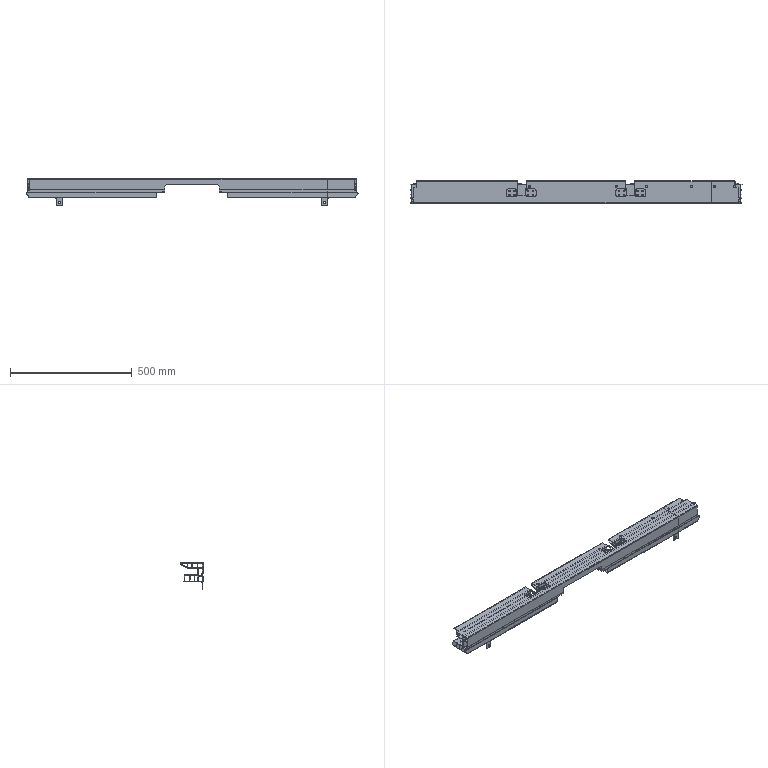NC program | NX | posted with a generic post | part box 1365 x 90.95 x 108.501 mm
Lines 1 to 1032 of 23380:
N10 G17 G21 G94 G90
(FLOOR_WALL_COPY_COPY , TOOL : D10)
N12 T10 M6
N14 G54
N16 G17 G0 G90 X-649.118 Y38.719 B0. C0. S6000 M3
N18 G43 Z30. H10
N20 Z0.524
N22 G94 G1 Z-0.976 F1000.
N24 X-648.541 Y39.719
N26 G2 X-647.675 Y40.219 R1.
N28 G1 X-622.6 F2500.
N30 Y44.
N32 G3 X-625. Y46.4 R2.4
N34 G1 X-658.759
N36 G2 X-658.96 Y46.442 R0.5
N38 G1 X-660.602 Y47.163
N40 X-660.976 Y47.3
N42 X-665.955 Y48.486
N44 G2 X-666.339 Y48.973 R0.5
N46 G1 Y57.612
N48 G2 X-665.945 Y58.1 R0.5
N50 G1 X-664.104 Y58.5
N52 X-672.75
N54 Y40.219
N56 X-647.675
N58 G2 X-646.809 Y39.719 R1.
N60 G1 X-646.232 Y38.719
N62 Z0.524
N64 G0 X-623.698
N66 G1 Z-0.976 F1000.
N68 X-622.6 Y39.353
N70 G3 X-622.1 Y40.219 R1.
N72 G1 Y44. F2500.
N74 G3 X-625. Y46.9 R2.9
N76 G1 X-658.759
N78 X-660.415 Y47.627
N80 X-660.832 Y47.779
N82 X-665.839 Y48.973
N84 Y57.612
N86 X-661.885 Y58.47
N88 G3 X-661.145 Y59.142 R1.
N90 G1 X-660.55 Y61.
N92 Z0.524
N94 G0 Z30.
N96 X-662.961 Y47.773
N98 Z0.524
N100 G1 X-666.007 Y48.502 Z0.36 F1000.
N102 X-666.045 Y48.515 Z0.358
N104 X-666.234 Y48.619 Z0.346
N106 X-666.339 Y48.797 Z0.335
N108 Y57.727 Z-0.133
N110 X-666.212 Y57.988 Z-0.148
N112 X-666.117 Y58.063 Z-0.154
N114 X-664.104 Y58.5 Z-0.262
N116 X-672.75 Z-0.715
N118 Y39.764 Z-1.697
N120 X-667.885 Z-1.952
N122 Y44.264
N124 X-667.52 F2500.
N126 G2 X-668.25 Y44.592 R5.
N128 G1 Y44.264
N130 X-667.885
N132 Y39.764
N134 X-622.6
N136 Y44.
N138 G3 X-625. Y46.4 R2.4
N140 G1 X-658.759
N142 G2 X-658.96 Y46.442 R0.5
N144 G1 X-660.602 Y47.163
N146 X-660.976 Y47.3
N148 X-666.007 Y48.502
N150 X-666.08 Y48.535
N152 G2 X-666.339 Y48.973 R0.5
N154 G1 Y57.612
N156 G2 X-665.945 Y58.1 R0.5
N158 G1 X-664.104 Y58.5
N160 X-672.75
N162 Y39.764
N164 X-667.885
N166 G2 X-667.019 Y39.264 R1.
N168 G1 X-666.442 Y38.264
N170 Z-0.452
N172 G0 X-623.698
N174 G1 Z-1.952 F1000.
N176 X-622.6 Y38.898
N178 G3 X-622.1 Y39.764 R1.
N180 G1 Y44. F2500.
N182 G3 X-625. Y46.9 R2.9
N184 G1 X-658.759
N186 X-660.415 Y47.627
N188 X-660.832 Y47.779
N190 X-665.839 Y48.973
N192 Y57.612
N194 X-661.885 Y58.47
N196 G3 X-661.145 Y59.142 R1.
N198 G1 X-660.55 Y61.
N200 Z-0.452
N202 G0 Z30.
N204 X-664.27 Y48.085
N206 Z-0.452
N208 G1 X-666.021 Y48.502 Z-0.546 F1000.
N210 X-666.234 Y48.619 Z-0.559
N212 X-666.339 Y48.797 Z-0.57
N214 Y57.727 Z-1.038
N216 X-666.212 Y57.988 Z-1.053
N218 X-666.117 Y58.063 Z-1.06
N220 X-664.104 Y58.5 Z-1.168
N222 X-672.75 Z-1.621
N224 Y39.309 Z-2.626
N226 X-666.995 Z-2.928
N228 Y43.809
N230 X-665.739 F2500.
N232 X-666.998 Y44.109
N234 G2 X-668.25 Y44.592 R5.
N236 G1 Y43.809
N238 X-666.995
N240 Y39.309
N242 X-622.6
N244 Y44.
N246 G3 X-625. Y46.4 R2.4
N248 G1 X-658.759
N250 G2 X-658.96 Y46.442 R0.5
N252 G1 X-660.602 Y47.163
N254 X-660.976 Y47.3
N256 X-665.955 Y48.486
N258 G2 X-666.339 Y48.973 R0.5
N260 G1 Y57.612
N262 G2 X-665.945 Y58.1 R0.5
N264 G1 X-664.104 Y58.5
N266 X-672.75
N268 Y39.309
N270 X-666.995
N272 G2 X-666.129 Y38.809 R1.
N274 G1 X-665.551 Y37.809
N276 Z-1.428
N278 G0 X-623.698
N280 G1 Z-2.928 F1000.
N282 X-622.6 Y38.443
N284 G3 X-622.1 Y39.309 R1.
N286 G1 Y44. F2500.
N288 G3 X-625. Y46.9 R2.9
N290 G1 X-658.759
N292 X-660.415 Y47.627
N294 X-660.832 Y47.779
N296 X-665.839 Y48.973
N298 Y57.612
N300 X-661.885 Y58.47
N302 G3 X-661.145 Y59.142 R1.
N304 G1 X-660.55 Y61.
N306 Z-1.428
N308 G0 Z30.
N310 X-665.665 Y43.791
N312 Z-1.428
N314 G1 X-667.532 Y44.236 Z-1.529 F1000.
N316 X-667.769 Y44.328 Z-1.542
N318 X-668.25 Y44.592 Z-1.571
N320 Y43.354 Z-1.636
N322 X-663.83 Z-1.867
N324 X-666.998 Y44.109 Z-2.038
N326 X-667.532 Y44.236 Z-2.067
N328 X-667.769 Y44.328 Z-2.08
N330 X-668.25 Y44.592 Z-2.109
N332 Y43.354 Z-2.174
N334 X-663.83 Z-2.405
N336 X-666.998 Y44.109 Z-2.576
N338 X-667.532 Y44.236 Z-2.605
N340 X-667.769 Y44.328 Z-2.618
N342 X-668.25 Y44.592 Z-2.647
N344 Y43.354 Z-2.712
N346 X-663.83 Z-2.944
N348 X-666.998 Y44.109 Z-3.114
N350 X-667.532 Y44.236 Z-3.143
N352 X-667.769 Y44.328 Z-3.156
N354 X-668.25 Y44.592 Z-3.185
N356 Y43.354 Z-3.25
N358 X-663.83 Z-3.482
N360 X-666.998 Y44.109 Z-3.652
N362 X-667.532 Y44.236 Z-3.681
N364 X-667.769 Y44.328 Z-3.694
N366 X-668.25 Y44.592 Z-3.723
N368 Y43.354 Z-3.788
N370 X-666.04 Z-3.904
N372 X-663.83 F2500.
N374 X-666.998 Y44.109
N376 G2 X-668.25 Y44.592 R5.
N378 G1 Y43.354
N380 X-666.04
N382 Y38.854
N384 X-622.6
N386 Y44.
N388 G3 X-625. Y46.4 R2.4
N390 G1 X-658.759
N392 G2 X-658.96 Y46.442 R0.5
N394 G1 X-660.602 Y47.163
N396 X-660.976 Y47.3
N398 X-665.955 Y48.486
N400 G2 X-666.339 Y48.973 R0.5
N402 G1 Y57.612
N404 G2 X-665.945 Y58.1 R0.5
N406 G1 X-664.104 Y58.5
N408 X-672.75
N410 Y38.854
N412 X-666.04
N414 G2 X-665.174 Y38.354 R1.
N416 G1 X-664.596 Y37.354
N418 Z-2.404
N420 G0 X-623.698
N422 G1 Z-3.904 F1000.
N424 X-622.6 Y37.988
N426 G3 X-622.1 Y38.854 R1.
N428 G1 Y44. F2500.
N430 G3 X-625. Y46.9 R2.9
N432 G1 X-658.759
N434 X-660.415 Y47.627
N436 X-660.832 Y47.779
N438 X-665.839 Y48.973
N440 Y57.612
N442 X-661.885 Y58.47
N444 G3 X-661.145 Y59.142 R1.
N446 G1 X-660.55 Y61.
N448 Z-2.404
N450 G0 Z30.
N452 X-668.25 Y44.222
N454 Z-2.404
N456 G1 Y42.899 Z-2.473 F1000.
N458 X-662.082 Z-2.797
N460 X-662.275 Y42.983 Z-2.808
N462 X-666.998 Y44.109 Z-3.062
N464 X-667.532 Y44.236 Z-3.091
N466 X-667.769 Y44.328 Z-3.104
N468 X-668.25 Y44.592 Z-3.133
N470 Y42.899 Z-3.222
N472 X-662.082 Z-3.545
N474 X-662.275 Y42.983 Z-3.556
N476 X-666.998 Y44.109 Z-3.81
N478 X-667.532 Y44.236 Z-3.839
N480 X-667.769 Y44.328 Z-3.852
N482 X-668.25 Y44.592 Z-3.881
N484 Y42.899 Z-3.97
N486 X-662.082 Z-4.293
N488 X-662.275 Y42.983 Z-4.304
N490 X-666.998 Y44.109 Z-4.559
N492 X-667.532 Y44.236 Z-4.587
N494 X-667.769 Y44.328 Z-4.601
N496 X-668.25 Y44.592 Z-4.629
N498 Y42.899 Z-4.718
N500 X-665.166 Z-4.88
N502 X-662.082 F2500.
N504 X-662.275 Y42.983
N506 X-666.998 Y44.109
N508 G2 X-668.25 Y44.592 R5.
N510 G1 Y42.899
N512 X-665.166
N514 Y38.399
N516 X-622.6
N518 Y44.
N520 G3 X-625. Y46.4 R2.4
N522 G1 X-658.759
N524 G2 X-658.96 Y46.442 R0.5
N526 G1 X-660.976 Y47.3
N528 X-665.955 Y48.486
N530 G2 X-666.339 Y48.973 R0.5
N532 G1 Y57.612
N534 G2 X-665.945 Y58.1 R0.5
N536 G1 X-664.104 Y58.5
N538 X-672.75
N540 Y38.399
N542 X-665.166
N544 G2 X-664.3 Y37.899 R1.
N546 G1 X-663.723 Y36.899
N548 Z-3.38
N550 G0 X-623.698
N552 G1 Z-4.88 F1000.
N554 X-622.6 Y37.533
N556 G3 X-622.1 Y38.399 R1.
N558 G1 Y44. F2500.
N560 G3 X-625. Y46.9 R2.9
N562 G1 X-658.759
N564 X-660.415 Y47.627
N566 X-660.832 Y47.779
N568 X-665.839 Y48.973
N570 Y57.612
N572 X-661.885 Y58.47
N574 G3 X-661.145 Y59.142 R1.
N576 G1 X-660.55 Y61.
N578 Z-3.38
N580 G0 Z30.
N582 X-661.184 Y42.444
N584 Z-3.38
N586 G1 X-661.046 Z-3.387 F1000.
N588 X-662.275 Y42.983 Z-3.457
N590 X-666.998 Y44.109 Z-3.712
N592 X-667.532 Y44.236 Z-3.741
N594 X-667.769 Y44.328 Z-3.754
N596 X-668.25 Y44.592 Z-3.783
N598 Y42.444 Z-3.895
N600 X-661.046 Z-4.273
N602 X-662.275 Y42.983 Z-4.343
N604 X-666.998 Y44.109 Z-4.598
N606 X-667.532 Y44.236 Z-4.627
N608 X-667.769 Y44.328 Z-4.64
N610 X-668.25 Y44.592 Z-4.669
N612 Y42.444 Z-4.781
N614 X-661.046 Z-5.159
N616 X-662.275 Y42.983 Z-5.229
N618 X-666.998 Y44.109 Z-5.484
N620 X-667.532 Y44.236 Z-5.512
N622 X-667.769 Y44.328 Z-5.526
N624 X-668.25 Y44.592 Z-5.554
N626 Y42.444 Z-5.667
N628 X-664.648 Z-5.856
N630 X-661.046 F2500.
N632 X-662.275 Y42.983
N634 X-666.998 Y44.109
N636 G2 X-668.25 Y44.592 R5.
N638 G1 Y42.444
N640 X-664.648
N642 Y37.944
N644 X-622.6
N646 Y44.
N648 G3 X-625. Y46.4 R2.4
N650 G1 X-658.759
N652 G2 X-658.96 Y46.442 R0.5
N654 G1 X-660.976 Y47.3
N656 X-665.955 Y48.486
N658 G2 X-666.339 Y48.973 R0.5
N660 G1 Y57.612
N662 G2 X-665.945 Y58.1 R0.5
N664 G1 X-664.104 Y58.5
N666 X-672.75
N668 Y37.944
N670 X-664.648
N672 G2 X-663.782 Y37.444 R1.
N674 G1 X-663.205 Y36.444
N676 Z-4.356
N678 G0 X-623.698
N680 G1 Z-5.856 F1000.
N682 X-622.6 Y37.078
N684 G3 X-622.1 Y37.944 R1.
N686 G1 Y44. F2500.
N688 G3 X-625. Y46.9 R2.9
N690 G1 X-658.759
N692 X-660.415 Y47.627
N694 X-660.832 Y47.779
N696 X-665.839 Y48.973
N698 Y57.612
N700 X-661.885 Y58.47
N702 G3 X-661.145 Y59.142 R1.
N704 G1 X-660.55 Y61.
N706 Z-4.356
N708 G0 Z30.
N710 X-668.182 Y44.555
N712 Z-4.356
N714 G1 X-668.25 Y44.592 Z-4.36 F1000.
N716 Y41.988 Z-4.496
N718 X-659.695 Z-4.945
N720 X-660.234 Y42.091 Z-4.973
N722 X-660.267 Y42.101 Z-4.975
N724 X-662.275 Y42.983 Z-5.09
N726 X-666.998 Y44.109 Z-5.345
N728 X-667.532 Y44.236 Z-5.373
N730 X-667.769 Y44.328 Z-5.387
N732 X-668.25 Y44.592 Z-5.415
N734 Y41.988 Z-5.552
N736 X-659.695 Z-6.
N738 X-660.234 Y42.091 Z-6.029
N740 X-660.267 Y42.101 Z-6.031
N742 X-662.275 Y42.983 Z-6.146
N744 X-666.998 Y44.109 Z-6.4
N746 X-667.532 Y44.236 Z-6.429
N748 X-667.769 Y44.328 Z-6.442
N750 X-668.25 Y44.592 Z-6.471
N752 Y41.988 Z-6.608
N754 X-663.973 Z-6.832
N756 X-659.695 F2500.
N758 G2 X-660.769 Y42.322 R5.
N760 G1 X-662.275 Y42.983
N762 X-666.998 Y44.109
N764 G2 X-668.25 Y44.592 R5.
N766 G1 Y41.988
N768 X-663.973
N770 Y37.488
N772 X-622.6
N774 Y44.
N776 G3 X-625. Y46.4 R2.4
N778 G1 X-658.759
N780 G2 X-658.96 Y46.442 R0.5
N782 G1 X-660.602 Y47.163
N784 X-660.976 Y47.3
N786 X-665.955 Y48.486
N788 G2 X-666.339 Y48.973 R0.5
N790 G1 Y57.612
N792 G2 X-665.945 Y58.1 R0.5
N794 G1 X-664.104 Y58.5
N796 X-672.75
N798 Y37.488
N800 X-663.973
N802 G2 X-663.107 Y36.988 R1.
N804 G1 X-662.529 Y35.988
N806 Z-5.332
N808 G0 X-623.698
N810 G1 Z-6.832 F1000.
N812 X-622.6 Y36.622
N814 G3 X-622.1 Y37.488 R1.
N816 G1 Y44. F2500.
N818 G3 X-625. Y46.9 R2.9
N820 G1 X-658.759
N822 X-660.415 Y47.627
N824 X-660.832 Y47.779
N826 X-665.839 Y48.973
N828 Y57.612
N830 X-661.885 Y58.47
N832 G3 X-661.145 Y59.142 R1.
N834 G1 X-660.55 Y61.
N836 Z-5.332
N838 G0 Z30.
N840 X-645.079 Y41.9
N842 Z-5.332
N844 G1 X-659.307 Z-6.077 F1000.
N846 X-660.267 Y42.101 Z-6.129
N848 X-662.275 Y42.983 Z-6.244
N850 X-666.998 Y44.109 Z-6.498
N852 X-667.532 Y44.236 Z-6.527
N854 X-667.769 Y44.328 Z-6.54
N856 X-668.25 Y44.592 Z-6.569
N858 Y41.533 Z-6.729
N860 X-647.675 Z-7.808
N862 X-627.1 F2500.
N864 Y41.9
N866 X-658.759
N868 G2 X-660.769 Y42.322 R5.
N870 G1 X-662.275 Y42.983
N872 X-666.998 Y44.109
N874 G2 X-668.25 Y44.592 R5.
N876 G1 Y41.533
N878 X-647.675
N880 Y37.033
N882 X-622.6
N884 Y44.
N886 G3 X-625. Y46.4 R2.4
N888 G1 X-658.759
N890 G2 X-658.96 Y46.442 R0.5
N892 G1 X-660.602 Y47.163
N894 X-660.976 Y47.3
N896 X-665.955 Y48.486
N898 G2 X-666.339 Y48.973 R0.5
N900 G1 Y57.612
N902 G2 X-665.945 Y58.1 R0.5
N904 G1 X-664.104 Y58.5
N906 X-672.75
N908 Y37.033
N910 X-647.675
N912 G2 X-646.809 Y36.533 R1.
N914 G1 X-646.232 Y35.533
N916 Z-6.308
N918 G0 X-623.698
N920 G1 Z-7.808 F1000.
N922 X-622.6 Y36.167
N924 G3 X-622.1 Y37.033 R1.
N926 G1 Y44. F2500.
N928 G3 X-625. Y46.9 R2.9
N930 G1 X-658.759
N932 X-660.415 Y47.627
N934 X-660.832 Y47.779
N936 X-665.839 Y48.973
N938 Y57.612
N940 X-661.885 Y58.47
N942 G3 X-661.145 Y59.142 R1.
N944 G1 X-660.55 Y61.
N946 Z-6.308
N948 G0 Z30.
N950 X-645.534 Y41.9
N952 Z-6.308
N954 G1 X-659.307 Z-7.029 F1000.
N956 X-660.267 Y42.101 Z-7.081
N958 X-662.275 Y42.983 Z-7.196
N960 X-666.998 Y44.109 Z-7.45
N962 X-667.532 Y44.236 Z-7.479
N964 X-667.769 Y44.328 Z-7.492
N966 X-668.25 Y44.592 Z-7.521
N968 Y41.078 Z-7.705
N970 X-647.675 Z-8.784
N972 X-627.1 F2500.
N974 Y41.9
N976 X-658.759
N978 G2 X-660.769 Y42.322 R5.
N980 G1 X-662.275 Y42.983
N982 X-666.998 Y44.109
N984 G2 X-668.25 Y44.592 R5.
N986 G1 Y41.078
N988 X-647.675
N990 Y36.578
N992 X-622.6
N994 Y44.
N996 G3 X-625. Y46.4 R2.4
N998 G1 X-658.759
N1000 G2 X-658.96 Y46.442 R0.5
N1002 G1 X-660.602 Y47.163
N1004 X-660.976 Y47.3
N1006 X-665.955 Y48.486
N1008 G2 X-666.339 Y48.973 R0.5
N1010 G1 Y57.612
N1012 G2 X-665.945 Y58.1 R0.5
N1014 G1 X-664.104 Y58.5
N1016 X-672.75
N1018 Y36.578
N1020 X-647.675
N1022 G2 X-646.809 Y36.078 R1.
N1024 G1 X-646.232 Y35.078
N1026 Z-7.284
N1028 G0 X-623.698
N1030 G1 Z-8.784 F1000.
N1032 X-622.6 Y35.712
N1034 G3 X-622.1 Y36.578 R1.
N1036 G1 Y44. F2500.
N1038 G3 X-625. Y46.9 R2.9
N1040 G1 X-658.759
N1042 X-660.415 Y47.627
N1044 X-660.832 Y47.779
N1046 X-665.839 Y48.973
N1048 Y57.612
N1050 X-661.885 Y58.47
N1052 G3 X-661.145 Y59.142 R1.
N1054 G1 X-660.55 Y61.
N1056 Z-7.284
N1058 G0 Z30.
N1060 X-645.989 Y41.9
N1062 Z-7.284
N1064 G1 X-659.307 Z-7.982 F1000.
N1066 X-660.267 Y42.101 Z-8.033
N1068 X-662.275 Y42.983 Z-8.148
N1070 X-666.998 Y44.109 Z-8.402
N1072 X-667.532 Y44.236 Z-8.431
N1074 X-667.769 Y44.328 Z-8.444
N1076 X-668.25 Y44.592 Z-8.473
N1078 Y40.623 Z-8.681
N1080 X-647.675 Z-9.759
N1082 X-627.1 F2500.
N1084 Y41.9
N1086 X-658.759
N1088 G2 X-660.769 Y42.322 R5.
N1090 G1 X-662.275 Y42.983
N1092 X-666.998 Y44.109
N1094 G2 X-668.25 Y44.592 R5.
N1096 G1 Y40.623
N1098 X-647.675
N1100 Y36.123
N1102 X-622.6
N1104 Y44.
N1106 G3 X-625. Y46.4 R2.4
N1108 G1 X-658.759
N1110 G2 X-658.96 Y46.442 R0.5
N1112 G1 X-660.602 Y47.163
N1114 X-660.976 Y47.3
N1116 X-665.955 Y48.486
N1118 G2 X-666.339 Y48.973 R0.5
N1120 G1 Y57.612
N1122 G2 X-665.945 Y58.1 R0.5
N1124 G1 X-664.104 Y58.5
N1126 X-672.75
N1128 Y36.123
N1130 X-647.675
N1132 G2 X-646.809 Y35.623 R1.
N1134 G1 X-646.232 Y34.623
N1136 Z-8.259
N1138 G0 X-623.698
N1140 G1 Z-9.759 F1000.
N1142 X-622.6 Y35.257
N1144 G3 X-622.1 Y36.123 R1.
N1146 G1 Y44. F2500.
N1148 G3 X-625. Y46.9 R2.9
N1150 G1 X-658.759
N1152 X-660.415 Y47.627
N1154 X-660.832 Y47.779
N1156 X-665.839 Y48.973
N1158 Y57.612
N1160 X-661.885 Y58.47
N1162 G3 X-661.145 Y59.142 R1.
N1164 G1 X-660.55 Y61.
N1166 Z-8.259
N1168 G0 Z30.
N1170 X-646.444 Y41.9
N1172 Z-8.259
N1174 G1 X-659.307 Z-8.934 F1000.
N1176 X-660.267 Y42.101 Z-8.985
N1178 X-662.275 Y42.983 Z-9.1
N1180 X-666.998 Y44.109 Z-9.354
N1182 X-667.532 Y44.236 Z-9.383
N1184 X-667.769 Y44.328 Z-9.396
N1186 X-668.25 Y44.592 Z-9.425
N1188 Y40.168 Z-9.657
N1190 X-647.675 Z-10.735
N1192 X-627.1 F2500.
N1194 Y41.9
N1196 X-658.759
N1198 G2 X-660.769 Y42.322 R5.
N1200 G1 X-662.275 Y42.983
N1202 X-666.998 Y44.109
N1204 G2 X-668.25 Y44.592 R5.
N1206 G1 Y40.168
N1208 X-647.675
N1210 Y35.668
N1212 X-622.6
N1214 Y44.
N1216 G3 X-625. Y46.4 R2.4
N1218 G1 X-658.759
N1220 G2 X-658.96 Y46.442 R0.5
N1222 G1 X-660.602 Y47.163
N1224 X-660.976 Y47.3
N1226 X-665.955 Y48.486
N1228 G2 X-666.339 Y48.973 R0.5
N1230 G1 Y57.612
N1232 G2 X-665.945 Y58.1 R0.5
N1234 G1 X-664.104 Y58.5
N1236 X-672.75
N1238 Y35.668
N1240 X-647.675
N1242 G2 X-646.809 Y35.168 R1.
N1244 G1 X-646.232 Y34.168
N1246 Z-9.235
N1248 G0 X-623.698
N1250 G1 Z-10.735 F1000.
N1252 X-622.6 Y34.802
N1254 G3 X-622.1 Y35.668 R1.
N1256 G1 Y44. F2500.
N1258 G3 X-625. Y46.9 R2.9
N1260 G1 X-658.759
N1262 X-660.415 Y47.627
N1264 X-660.832 Y47.779
N1266 X-665.839 Y48.973
N1268 Y57.612
N1270 X-661.885 Y58.47
N1272 G3 X-661.145 Y59.142 R1.
N1274 G1 X-660.55 Y61.
N1276 Z-9.235
N1278 G0 Z30.
N1280 X-646.899 Y41.9
N1282 Z-9.235
N1284 G1 X-659.307 Z-9.886 F1000.
N1286 X-660.267 Y42.101 Z-9.937
N1288 X-662.275 Y42.983 Z-10.052
N1290 X-666.998 Y44.109 Z-10.306
N1292 X-667.532 Y44.236 Z-10.335
N1294 X-667.769 Y44.328 Z-10.349
N1296 X-668.25 Y44.592 Z-10.377
N1298 Y39.713 Z-10.633
N1300 X-647.675 Z-11.711
N1302 X-627.1 F2500.
N1304 Y41.9
N1306 X-658.759
N1308 G2 X-660.769 Y42.322 R5.
N1310 G1 X-662.275 Y42.983
N1312 X-666.998 Y44.109
N1314 G2 X-668.25 Y44.592 R5.
N1316 G1 Y39.713
N1318 X-647.675
N1320 Y35.213
N1322 X-622.6
N1324 Y44.
N1326 G3 X-625. Y46.4 R2.4
N1328 G1 X-658.759
N1330 G2 X-658.96 Y46.442 R0.5
N1332 G1 X-660.602 Y47.163
N1334 X-660.976 Y47.3
N1336 X-665.955 Y48.486
N1338 G2 X-666.339 Y48.973 R0.5
N1340 G1 Y57.612
N1342 G2 X-665.945 Y58.1 R0.5
N1344 G1 X-664.104 Y58.5
N1346 X-672.75
N1348 Y35.213
N1350 X-647.675
N1352 G2 X-646.809 Y34.713 R1.
N1354 G1 X-646.232 Y33.713
N1356 Z-10.211
N1358 G0 X-623.698
N1360 G1 Z-11.711 F1000.
N1362 X-622.6 Y34.347
N1364 G3 X-622.1 Y35.213 R1.
N1366 G1 Y44. F2500.
N1368 G3 X-625. Y46.9 R2.9
N1370 G1 X-658.759
N1372 X-660.415 Y47.627
N1374 X-660.832 Y47.779
N1376 X-665.839 Y48.973
N1378 Y57.612
N1380 X-661.885 Y58.47
N1382 G3 X-661.145 Y59.142 R1.
N1384 G1 X-660.55 Y61.
N1386 Z-10.211
N1388 G0 Z30.
N1390 X-647.354 Y41.9
N1392 Z-10.211
N1394 G1 X-659.307 Z-10.838 F1000.
N1396 X-660.267 Y42.101 Z-10.889
N1398 X-662.275 Y42.983 Z-11.004
N1400 X-666.998 Y44.109 Z-11.259
N1402 X-667.532 Y44.236 Z-11.287
N1404 X-667.769 Y44.328 Z-11.301
N1406 X-668.25 Y44.592 Z-11.329
N1408 Y39.258 Z-11.609
N1410 X-647.675 Z-12.687
N1412 X-627.1 F2500.
N1414 Y41.9
N1416 X-658.759
N1418 G2 X-660.769 Y42.322 R5.
N1420 G1 X-662.275 Y42.983
N1422 X-666.998 Y44.109
N1424 G2 X-668.25 Y44.592 R5.
N1426 G1 Y39.258
N1428 X-647.675
N1430 Y34.758
N1432 X-622.6
N1434 Y44.
N1436 G3 X-625. Y46.4 R2.4
N1438 G1 X-658.759
N1440 G2 X-658.96 Y46.442 R0.5
N1442 G1 X-660.602 Y47.163
N1444 X-660.976 Y47.3
N1446 X-665.955 Y48.486
N1448 G2 X-666.339 Y48.973 R0.5
N1450 G1 Y57.612
N1452 G2 X-665.945 Y58.1 R0.5
N1454 G1 X-664.104 Y58.5
N1456 X-672.75
N1458 Y34.758
N1460 X-647.675
N1462 G2 X-646.809 Y34.258 R1.
N1464 G1 X-646.232 Y33.258
N1466 Z-11.187
N1468 G0 X-623.698
N1470 G1 Z-12.687 F1000.
N1472 X-622.6 Y33.892
N1474 G3 X-622.1 Y34.758 R1.
N1476 G1 Y44. F2500.
N1478 G3 X-625. Y46.9 R2.9
N1480 G1 X-658.759
N1482 X-660.415 Y47.627
N1484 X-660.832 Y47.779
N1486 X-665.839 Y48.973
N1488 Y57.612
N1490 X-661.885 Y58.47
N1492 G3 X-661.145 Y59.142 R1.
N1494 G1 X-660.55 Y61.
N1496 Z-11.187
N1498 G0 Z30.
N1500 X-647.809 Y41.9
N1502 Z-11.187
N1504 G1 X-659.307 Z-11.79 F1000.
N1506 X-660.267 Y42.101 Z-11.841
N1508 X-662.275 Y42.983 Z-11.956
N1510 X-666.998 Y44.109 Z-12.211
N1512 X-667.532 Y44.236 Z-12.239
N1514 X-667.769 Y44.328 Z-12.253
N1516 X-668.25 Y44.592 Z-12.281
N1518 Y38.803 Z-12.585
N1520 X-647.675 Z-13.663
N1522 X-627.1 F2500.
N1524 Y41.9
N1526 X-658.759
N1528 G2 X-660.769 Y42.322 R5.
N1530 G1 X-662.275 Y42.983
N1532 X-666.998 Y44.109
N1534 G2 X-668.25 Y44.592 R5.
N1536 G1 Y38.803
N1538 X-647.675
N1540 Y34.303
N1542 X-622.6
N1544 Y44.
N1546 G3 X-625. Y46.4 R2.4
N1548 G1 X-658.759
N1550 G2 X-658.96 Y46.442 R0.5
N1552 G1 X-660.602 Y47.163
N1554 X-660.976 Y47.3
N1556 X-665.955 Y48.486
N1558 G2 X-666.339 Y48.973 R0.5
N1560 G1 Y57.612
N1562 G2 X-665.945 Y58.1 R0.5
N1564 G1 X-664.104 Y58.5
N1566 X-672.75
N1568 Y34.303
N1570 X-647.675
N1572 G2 X-646.809 Y33.803 R1.
N1574 G1 X-646.232 Y32.803
N1576 Z-12.163
N1578 G0 X-623.698
N1580 G1 Z-13.663 F1000.
N1582 X-622.6 Y33.437
N1584 G3 X-622.1 Y34.303 R1.
N1586 G1 Y44. F2500.
N1588 G3 X-625. Y46.9 R2.9
N1590 G1 X-658.759
N1592 X-660.415 Y47.627
N1594 X-660.832 Y47.779
N1596 X-665.839 Y48.973
N1598 Y57.612
N1600 X-661.885 Y58.47
N1602 G3 X-661.145 Y59.142 R1.
N1604 G1 X-660.55 Y61.
N1606 Z-12.163
N1608 G0 X-666.406 Z-13.139
N1610 G1 Z-14.639 F1000.
N1612 X-667.561 Y59.
N1614 G2 X-668.427 Y58.5 R1.
N1616 G1 X-672.75 F2500.
N1618 Y47.5
N1620 X-661.817
N1622 X-665.955 Y48.486
N1624 G2 X-666.339 Y48.973 R0.5
N1626 G1 Y57.612
N1628 G2 X-665.945 Y58.1 R0.5
N1630 G1 X-664.104 Y58.5
N1632 X-668.427
N1634 G2 X-669.293 Y59. R1.
N1636 G1 X-670.448 Y61.
N1638 Z-13.139
N1640 G0 Z30.
N1642 X-665.839 Y53.123
N1644 Z-12.163
N1646 G1 Y48.973 Z-12.381 F1000.
N1648 X-660.832 Y47.779 Z-12.65
N1650 X-660.415 Y47.627 Z-12.674
N1652 X-660.125 Y47.5 Z-12.69
N1654 X-660.415 Y47.627 Z-12.707
N1656 X-660.832 Y47.779 Z-12.73
N1658 X-665.839 Y48.973 Z-13.
N1660 Y57.612 Z-13.453
N1662 X-661.885 Y58.47 Z-13.665
N1664 X-665.839 Y57.612 Z-13.877
N1666 Y48.973 Z-14.329
N1668 X-660.832 Y47.779 Z-14.599
N1670 X-660.415 Y47.627 Z-14.622
N1672 X-660.125 Y47.5 Z-14.639
N1674 X-660.415 Y47.627 F2500.
N1676 X-660.832 Y47.779
N1678 X-665.839 Y48.973
N1680 Y57.612
N1682 X-661.885 Y58.47
N1684 G3 X-661.145 Y59.142 R1.
N1686 G1 X-660.55 Y61.
N1688 Z-13.139
N1690 G0 X-666.406 Z-14.115
N1692 G1 Z-15.615 F1000.
N1694 X-667.561 Y59.
N1696 G2 X-668.427 Y58.5 R1.
N1698 G1 X-672.75 F2500.
N1700 Y47.5
N1702 X-661.817
N1704 X-665.955 Y48.486
N1706 G2 X-666.339 Y48.973 R0.5
N1708 G1 Y57.612
N1710 G2 X-665.945 Y58.1 R0.5
N1712 G1 X-664.104 Y58.5
N1714 X-668.427
N1716 G2 X-669.293 Y59. R1.
N1718 G1 X-670.448 Y61.
N1720 Z-14.115
N1722 G0 Z30.
N1724 X-665.839 Y53.123
N1726 Z-13.139
N1728 G1 Y48.973 Z-13.357 F1000.
N1730 X-660.832 Y47.779 Z-13.626
N1732 X-660.415 Y47.627 Z-13.65
N1734 X-660.125 Y47.5 Z-13.666
N1736 X-660.415 Y47.627 Z-13.683
N1738 X-660.832 Y47.779 Z-13.706
N1740 X-665.839 Y48.973 Z-13.976
N1742 Y57.612 Z-14.428
N1744 X-661.885 Y58.47 Z-14.641
N1746 X-665.839 Y57.612 Z-14.853
N1748 Y48.973 Z-15.305
N1750 X-660.832 Y47.779 Z-15.575
N1752 X-660.415 Y47.627 Z-15.598
N1754 X-660.125 Y47.5 Z-15.615
N1756 X-660.415 Y47.627 F2500.
N1758 X-660.832 Y47.779
N1760 X-665.839 Y48.973
N1762 Y57.612
N1764 X-661.885 Y58.47
N1766 G3 X-661.145 Y59.142 R1.
N1768 G1 X-660.55 Y61.
N1770 Z-14.115
N1772 G0 X-666.406 Z-15.091
N1774 G1 Z-16.591 F1000.
N1776 X-667.561 Y59.
N1778 G2 X-668.427 Y58.5 R1.
N1780 G1 X-672.75 F2500.
N1782 Y47.5
N1784 X-661.817
N1786 X-665.955 Y48.486
N1788 G2 X-666.339 Y48.973 R0.5
N1790 G1 Y57.612
N1792 G2 X-665.945 Y58.1 R0.5
N1794 G1 X-664.104 Y58.5
N1796 X-668.427
N1798 G2 X-669.293 Y59. R1.
N1800 G1 X-670.448 Y61.
N1802 Z-15.091
N1804 G0 Z30.
N1806 X-665.839 Y53.123
N1808 Z-14.115
N1810 G1 Y48.973 Z-14.332 F1000.
N1812 X-660.832 Y47.779 Z-14.602
N1814 X-660.415 Y47.627 Z-14.625
N1816 X-660.125 Y47.5 Z-14.642
N1818 X-660.415 Y47.627 Z-14.659
N1820 X-660.832 Y47.779 Z-14.682
N1822 X-665.839 Y48.973 Z-14.952
N1824 Y57.612 Z-15.404
N1826 X-661.885 Y58.47 Z-15.616
N1828 X-665.839 Y57.612 Z-15.828
N1830 Y48.973 Z-16.281
N1832 X-660.832 Y47.779 Z-16.551
N1834 X-660.415 Y47.627 Z-16.574
N1836 X-660.125 Y47.5 Z-16.591
N1838 X-660.415 Y47.627 F2500.
N1840 X-660.832 Y47.779
N1842 X-665.839 Y48.973
N1844 Y57.612
N1846 X-661.885 Y58.47
N1848 G3 X-661.145 Y59.142 R1.
N1850 G1 X-660.55 Y61.
N1852 Z-15.091
N1854 G0 X-666.406 Z-16.067
N1856 G1 Z-17.567 F1000.
N1858 X-667.561 Y59.
N1860 G2 X-668.427 Y58.5 R1.
N1862 G1 X-672.75 F2500.
N1864 Y47.5
N1866 X-661.817
N1868 X-665.955 Y48.486
N1870 G2 X-666.339 Y48.973 R0.5
N1872 G1 Y57.612
N1874 G2 X-665.945 Y58.1 R0.5
N1876 G1 X-664.104 Y58.5
N1878 X-668.427
N1880 G2 X-669.293 Y59. R1.
N1882 G1 X-670.448 Y61.
N1884 Z-16.067
N1886 G0 Z30.
N1888 X-665.839 Y53.123
N1890 Z-15.091
N1892 G1 Y48.973 Z-15.308 F1000.
N1894 X-660.832 Y47.779 Z-15.578
N1896 X-660.415 Y47.627 Z-15.601
N1898 X-660.125 Y47.5 Z-15.618
N1900 X-660.415 Y47.627 Z-15.635
N1902 X-660.832 Y47.779 Z-15.658
N1904 X-665.839 Y48.973 Z-15.928
N1906 Y57.612 Z-16.38
N1908 X-661.885 Y58.47 Z-16.592
N1910 X-665.839 Y57.612 Z-16.804
N1912 Y48.973 Z-17.257
N1914 X-660.832 Y47.779 Z-17.527
N1916 X-660.415 Y47.627 Z-17.55
N1918 X-660.125 Y47.5 Z-17.567
N1920 X-660.415 Y47.627 F2500.
N1922 X-660.832 Y47.779
N1924 X-665.839 Y48.973
N1926 Y57.612
N1928 X-661.885 Y58.47
N1930 G3 X-661.145 Y59.142 R1.
N1932 G1 X-660.55 Y61.
N1934 Z-16.067
N1936 G0 X-666.406 Z-17.043
N1938 G1 Z-18.543 F1000.
N1940 X-667.561 Y59.
N1942 G2 X-668.427 Y58.5 R1.
N1944 G1 X-672.75 F2500.
N1946 Y47.5
N1948 X-661.817
N1950 X-665.955 Y48.486
N1952 G2 X-666.339 Y48.973 R0.5
N1954 G1 Y57.612
N1956 G2 X-665.945 Y58.1 R0.5
N1958 G1 X-664.104 Y58.5
N1960 X-668.427
N1962 G2 X-669.293 Y59. R1.
N1964 G1 X-670.448 Y61.
N1966 Z-17.043
N1968 G0 Z30.
N1970 X-658.831 Y46.741
N1972 Z-17.043
N1974 G1 Z-18.543 F1000.
N1976 X-659.533 Y46.694
N1978 G3 X-660.125 Y47.5 R1.
N1980 G1 X-660.415 Y47.627 F2500.
N1982 X-660.832 Y47.779
N1984 X-665.839 Y48.973
N1986 Y57.612
N1988 X-661.885 Y58.47
N1990 G3 X-661.145 Y59.142 R1.
N1992 G1 X-660.55 Y61.
N1994 Z-17.043
N1996 G0 X-666.406 Z-18.019
N1998 G1 Z-19.519 F1000.
N2000 X-667.561 Y59.
N2002 G2 X-668.427 Y58.5 R1.
N2004 G1 X-672.75 F2500.
N2006 Y47.5
N2008 X-661.817
N2010 X-665.955 Y48.486
N2012 G2 X-666.339 Y48.973 R0.5
N2014 G1 Y57.612
N2016 G2 X-665.945 Y58.1 R0.5
N2018 G1 X-664.104 Y58.5
N2020 X-668.427
N2022 G2 X-669.293 Y59. R1.
N2024 G1 X-670.448 Y61.
N2026 Z-18.019
N2028 G0 Z30.
N2030 X-659.237 Y46.291
N2032 Z-18.019
N2034 G1 Z-19.519 F1000.
N2036 X-659.533 Y46.694
N2038 G3 X-660.125 Y47.5 R1.
N2040 G1 X-660.415 Y47.627 F2500.
N2042 X-660.832 Y47.779
N2044 X-665.839 Y48.973
N2046 Y57.612
N2048 X-661.885 Y58.47
N2050 G3 X-661.145 Y59.142 R1.
N2052 G1 X-660.55 Y61.
N2054 Z-18.019
N2056 G0 X-666.406 Z-18.995
N2058 G1 Z-20.495 F1000.
N2060 X-667.561 Y59.
N2062 G2 X-668.427 Y58.5 R1.